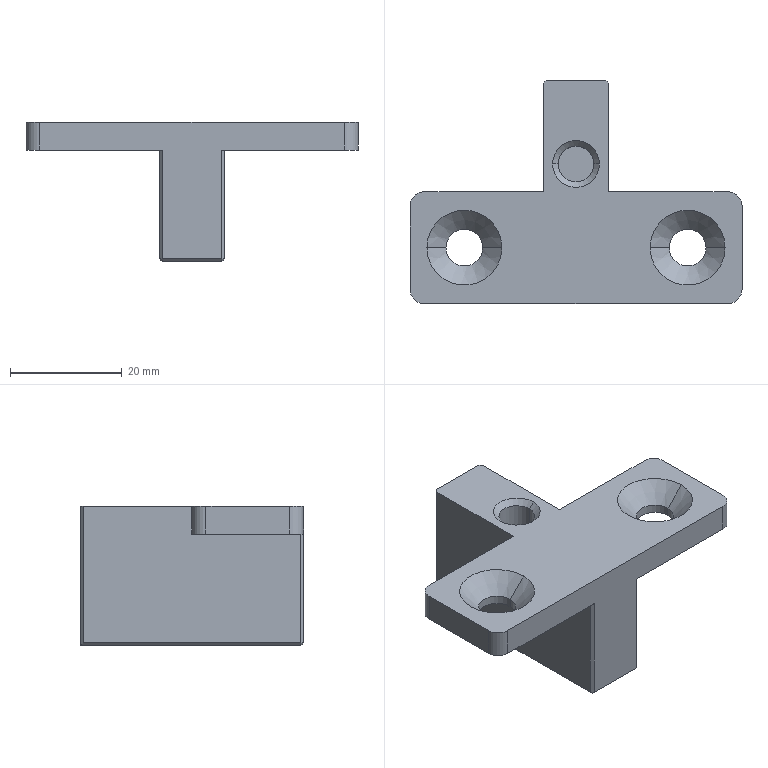Part | STEP file | 1 solid | 38 faces | box 59.5 x 40 x 25 mm | volume 15043 mm3 | plane 22 | cylinder 10 | cone 6 | commonest cylinder face diameters 5 x4 6.6 x4 6.4 x2